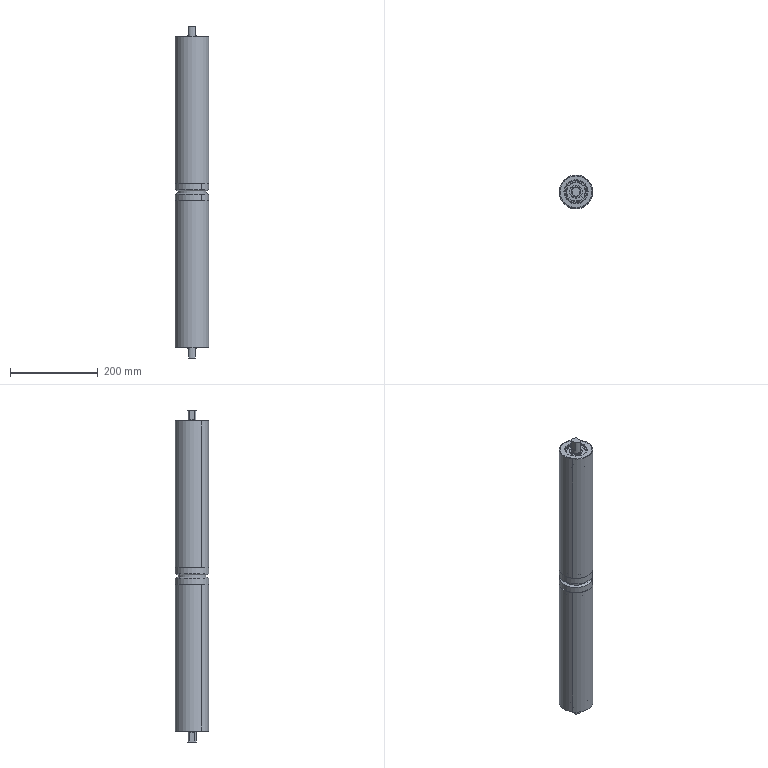Part | SolidWorks | features MirrorCompFeat 1 | 32 solids | 230 faces | box 76 x 76 x 755 mm | volume 913977 mm3 | cylinder 106 | spline 64 | plane 56 | cone 4 | commonest cylinder face diameters 28.4 x16 44.6 x16 52 x12 72 x12 20 x10 30.2 x8